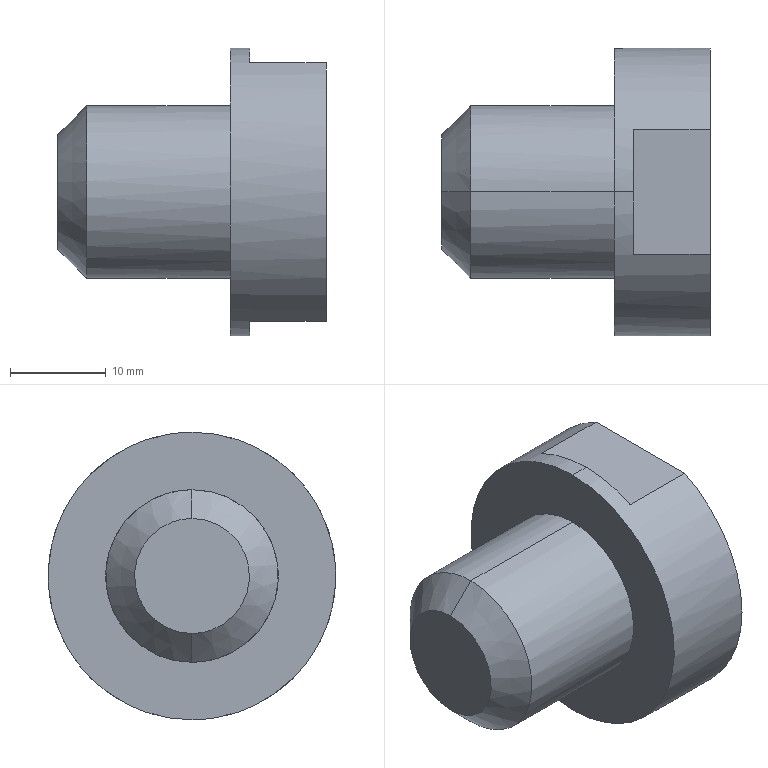Part | SolidWorks | features BaseBody 1 | 1 solid | 19 faces | box 28 x 30 x 30 mm | volume 9162 mm3 | plane 7 | cone 6 | cylinder 6 | commonest cylinder face diameters 10.106 x2 18 x2 30 x2
STEP:
#1=CARTESIAN_POINT('',(26.5,0.,5.053));
#2=VERTEX_POINT('',#1);
#3=CARTESIAN_POINT('',(26.5,0.,-5.053));
#4=VERTEX_POINT('',#3);
#5=CARTESIAN_POINT('',(26.5,0.,5.053));
#6=CARTESIAN_POINT('',(26.5,-0.6614,5.053));
#7=CARTESIAN_POINT('',(26.5,-1.323,4.921));
#8=CARTESIAN_POINT('',(26.5,-2.545,4.415));
#9=CARTESIAN_POINT('',(26.5,-3.105,4.041));
#10=CARTESIAN_POINT('',(26.5,-4.041,3.105));
#11=CARTESIAN_POINT('',(26.5,-4.415,2.545));
#12=CARTESIAN_POINT('',(26.5,-4.921,1.323));
#13=CARTESIAN_POINT('',(26.5,-5.053,0.6614));
#14=CARTESIAN_POINT('',(26.5,-5.053,-0.6614));
#15=CARTESIAN_POINT('',(26.5,-4.921,-1.323));
#16=CARTESIAN_POINT('',(26.5,-4.415,-2.545));
#17=CARTESIAN_POINT('',(26.5,-4.041,-3.105));
#18=CARTESIAN_POINT('',(26.5,-3.105,-4.041));
#19=CARTESIAN_POINT('',(26.5,-2.545,-4.415));
#20=CARTESIAN_POINT('',(26.5,-1.323,-4.921));
#21=CARTESIAN_POINT('',(26.5,-0.6614,-5.053));
#22=CARTESIAN_POINT('',(26.5,0.,-5.053));
#23=B_SPLINE_CURVE_WITH_KNOTS('',3,(#5,#6,#7,#8,#9,#10,#11,#12,#13,#14,#15,#16,#17,#18,#19,#20,#21,#22),.UNSPECIFIED.,.F.,.F.,(4,2,2,2,2,2,2,2,4),(3.142,3.534,3.927,4.32,4.712,5.105,5.498,5.89,6.283),.UNSPECIFIED.);
#24=EDGE_CURVE('',#2,#4,#23,.T.);
#25=ORIENTED_EDGE('',*,*,#24,.F.);
#26=CARTESIAN_POINT('',(28.,0.,6.553));
#27=VERTEX_POINT('',#26);
#28=CARTESIAN_POINT('',(26.5,0.,5.053));
#29=DIRECTION('',(0.7071,0.,0.7071));
#30=VECTOR('',#29,1000.);
#31=LINE('',#28,#30);
#32=EDGE_CURVE('',#2,#27,#31,.T.);
#33=ORIENTED_EDGE('',*,*,#32,.T.);
#34=CARTESIAN_POINT('',(28.,0.,-6.553));
#35=VERTEX_POINT('',#34);
#36=CARTESIAN_POINT('',(28.,0.,6.553));
#37=CARTESIAN_POINT('',(28.,-0.8578,6.553));
#38=CARTESIAN_POINT('',(28.,-1.715,6.382));
#39=CARTESIAN_POINT('',(28.,-3.3,5.726));
#40=CARTESIAN_POINT('',(28.,-4.027,5.24));
#41=CARTESIAN_POINT('',(28.,-5.24,4.027));
#42=CARTESIAN_POINT('',(28.,-5.726,3.3));
#43=CARTESIAN_POINT('',(28.,-6.382,1.715));
#44=CARTESIAN_POINT('',(28.,-6.553,0.8578));
#45=CARTESIAN_POINT('',(28.,-6.553,-0.8578));
#46=CARTESIAN_POINT('',(28.,-6.382,-1.715));
#47=CARTESIAN_POINT('',(28.,-5.726,-3.3));
#48=CARTESIAN_POINT('',(28.,-5.24,-4.027));
#49=CARTESIAN_POINT('',(28.,-4.027,-5.24));
#50=CARTESIAN_POINT('',(28.,-3.3,-5.726));
#51=CARTESIAN_POINT('',(28.,-1.715,-6.382));
#52=CARTESIAN_POINT('',(28.,-0.8578,-6.553));
#53=CARTESIAN_POINT('',(28.,0.,-6.553));
#54=B_SPLINE_CURVE_WITH_KNOTS('',3,(#36,#37,#38,#39,#40,#41,#42,#43,#44,#45,#46,#47,#48,#49,#50,#51,#52,#53),.UNSPECIFIED.,.F.,.F.,(4,2,2,2,2,2,2,2,4),(3.142,3.534,3.927,4.32,4.712,5.105,5.498,5.89,6.283),.UNSPECIFIED.);
#55=EDGE_CURVE('',#27,#35,#54,.T.);
#56=ORIENTED_EDGE('',*,*,#55,.T.);
#57=CARTESIAN_POINT('',(26.5,0.,-5.053));
#58=DIRECTION('',(0.7071,0.,-0.7071));
#59=VECTOR('',#58,1000.);
#60=LINE('',#57,#59);
#61=EDGE_CURVE('',#4,#35,#60,.T.);
#62=ORIENTED_EDGE('',*,*,#61,.F.);
#63=EDGE_LOOP('',(#25,#33,#56,#62));
#64=FACE_OUTER_BOUND('',#63,.T.);
#65=CARTESIAN_POINT('',(26.5,0.,0.));
#66=DIRECTION('',(1.,0.,0.));
#67=DIRECTION('',(0.,0.,-1.));
#68=AXIS2_PLACEMENT_3D('',#65,#66,#67);
#69=CONICAL_SURFACE('',#68,5.053,0.7854);
#70=ADVANCED_FACE('',(#64),#69,.F.);
#71=CARTESIAN_POINT('',(3.917,0.,5.053));
#72=VERTEX_POINT('',#71);
#73=CARTESIAN_POINT('',(3.917,0.,-5.053));
#74=VERTEX_POINT('',#73);
#75=CARTESIAN_POINT('',(3.917,0.,5.053));
#76=CARTESIAN_POINT('',(3.917,-0.6614,5.053));
#77=CARTESIAN_POINT('',(3.917,-1.323,4.921));
#78=CARTESIAN_POINT('',(3.917,-2.545,4.415));
#79=CARTESIAN_POINT('',(3.917,-3.105,4.041));
#80=CARTESIAN_POINT('',(3.917,-4.041,3.105));
#81=CARTESIAN_POINT('',(3.917,-4.415,2.545));
#82=CARTESIAN_POINT('',(3.917,-4.921,1.323));
#83=CARTESIAN_POINT('',(3.917,-5.053,0.6614));
#84=CARTESIAN_POINT('',(3.917,-5.053,-0.6614));
#85=CARTESIAN_POINT('',(3.917,-4.921,-1.323));
#86=CARTESIAN_POINT('',(3.917,-4.415,-2.545));
#87=CARTESIAN_POINT('',(3.917,-4.041,-3.105));
#88=CARTESIAN_POINT('',(3.917,-3.105,-4.041));
#89=CARTESIAN_POINT('',(3.917,-2.545,-4.415));
#90=CARTESIAN_POINT('',(3.917,-1.323,-4.921));
#91=CARTESIAN_POINT('',(3.917,-0.6614,-5.053));
#92=CARTESIAN_POINT('',(3.917,0.,-5.053));
#93=B_SPLINE_CURVE_WITH_KNOTS('',3,(#75,#76,#77,#78,#79,#80,#81,#82,#83,#84,#85,#86,#87,#88,#89,#90,#91,#92),.UNSPECIFIED.,.F.,.F.,(4,2,2,2,2,2,2,2,4),(3.142,3.534,3.927,4.32,4.712,5.105,5.498,5.89,6.283),.UNSPECIFIED.);
#94=EDGE_CURVE('',#72,#74,#93,.T.);
#95=ORIENTED_EDGE('',*,*,#94,.F.);
#96=CARTESIAN_POINT('',(28.,0.,5.053));
#97=DIRECTION('',(1.,0.,0.));
#98=VECTOR('',#97,1000.);
#99=LINE('',#96,#98);
#100=EDGE_CURVE('',#72,#2,#99,.T.);
#101=ORIENTED_EDGE('',*,*,#100,.T.);
#102=ORIENTED_EDGE('',*,*,#24,.T.);
#103=CARTESIAN_POINT('',(28.,0.,-5.053));
#104=DIRECTION('',(1.,0.,0.));
#105=VECTOR('',#104,1000.);
#106=LINE('',#103,#105);
#107=EDGE_CURVE('',#74,#4,#106,.T.);
#108=ORIENTED_EDGE('',*,*,#107,.F.);
#109=EDGE_LOOP('',(#95,#101,#102,#108));
#110=FACE_OUTER_BOUND('',#109,.T.);
#111=CARTESIAN_POINT('',(28.,0.,0.));
#112=DIRECTION('',(1.,0.,0.));
#113=DIRECTION('',(0.,0.,-1.));
#114=AXIS2_PLACEMENT_3D('',#111,#112,#113);
#115=CYLINDRICAL_SURFACE('',#114,5.053);
#116=ADVANCED_FACE('',(#110),#115,.F.);
#117=CARTESIAN_POINT('',(1.,0.,0.));
#118=VERTEX_POINT('',#117);
#119=CARTESIAN_POINT('',(1.,0.,0.));
#120=DIRECTION('',(0.5,0.,-0.866));
#121=VECTOR('',#120,1000.);
#122=LINE('',#119,#121);
#123=EDGE_CURVE('',#118,#74,#122,.T.);
#124=ORIENTED_EDGE('',*,*,#123,.F.);
#125=CARTESIAN_POINT('',(1.,0.,0.));
#126=DIRECTION('',(0.5,0.,0.866));
#127=VECTOR('',#126,1000.);
#128=LINE('',#125,#127);
#129=EDGE_CURVE('',#118,#72,#128,.T.);
#130=ORIENTED_EDGE('',*,*,#129,.T.);
#131=ORIENTED_EDGE('',*,*,#94,.T.);
#132=EDGE_LOOP('',(#124,#130,#131));
#133=FACE_OUTER_BOUND('',#132,.T.);
#134=CARTESIAN_POINT('',(1001.,0.,0.));
#135=DIRECTION('',(1.,0.,0.));
#136=DIRECTION('',(0.,0.,-1.));
#137=AXIS2_PLACEMENT_3D('',#134,#135,#136);
#138=CONICAL_SURFACE('',#137,1732.051,1.047);
#139=ADVANCED_FACE('',(#133),#138,.F.);
#140=CARTESIAN_POINT('',(3.,0.,-9.));
#141=VERTEX_POINT('',#140);
#142=CARTESIAN_POINT('',(3.,0.,9.));
#143=VERTEX_POINT('',#142);
#144=CARTESIAN_POINT('',(3.,0.,-9.));
#145=CARTESIAN_POINT('',(3.,1.178,-9.));
#146=CARTESIAN_POINT('',(3.,2.356,-8.766));
#147=CARTESIAN_POINT('',(3.,4.533,-7.864));
#148=CARTESIAN_POINT('',(3.,5.531,-7.197));
#149=CARTESIAN_POINT('',(3.,7.197,-5.531));
#150=CARTESIAN_POINT('',(3.,7.864,-4.533));
#151=CARTESIAN_POINT('',(3.,8.766,-2.356));
#152=CARTESIAN_POINT('',(3.,9.,-1.178));
#153=CARTESIAN_POINT('',(3.,9.,1.178));
#154=CARTESIAN_POINT('',(3.,8.766,2.356));
#155=CARTESIAN_POINT('',(3.,7.864,4.533));
#156=CARTESIAN_POINT('',(3.,7.197,5.531));
#157=CARTESIAN_POINT('',(3.,5.531,7.197));
#158=CARTESIAN_POINT('',(3.,4.533,7.864));
#159=CARTESIAN_POINT('',(3.,2.356,8.766));
#160=CARTESIAN_POINT('',(3.,1.178,9.));
#161=CARTESIAN_POINT('',(3.,0.,9.));
#162=B_SPLINE_CURVE_WITH_KNOTS('',3,(#144,#145,#146,#147,#148,#149,#150,#151,#152,#153,#154,#155,#156,#157,#158,#159,#160,#161),.UNSPECIFIED.,.F.,.F.,(4,2,2,2,2,2,2,2,4),(0.,0.3927,0.7854,1.178,1.571,1.963,2.356,2.749,3.142),.UNSPECIFIED.);
#163=EDGE_CURVE('',#141,#143,#162,.T.);
#164=ORIENTED_EDGE('',*,*,#163,.T.);
#165=CARTESIAN_POINT('',(18.,0.,9.));
#166=VERTEX_POINT('',#165);
#167=CARTESIAN_POINT('',(28.,0.,9.));
#168=DIRECTION('',(1.,0.,0.));
#169=VECTOR('',#168,1000.);
#170=LINE('',#167,#169);
#171=EDGE_CURVE('',#143,#166,#170,.T.);
#172=ORIENTED_EDGE('',*,*,#171,.T.);
#173=CARTESIAN_POINT('',(18.,0.,-9.));
#174=VERTEX_POINT('',#173);
#175=CARTESIAN_POINT('',(18.,0.,-9.));
#176=CARTESIAN_POINT('',(18.,0.5909,-9.));
#177=CARTESIAN_POINT('',(18.,1.176,-8.942));
#178=CARTESIAN_POINT('',(18.,2.335,-8.712));
#179=CARTESIAN_POINT('',(18.,2.898,-8.541));
#180=CARTESIAN_POINT('',(18.,3.99,-8.089));
#181=CARTESIAN_POINT('',(18.,4.509,-7.812));
#182=CARTESIAN_POINT('',(18.,5.491,-7.155));
#183=CARTESIAN_POINT('',(18.,5.946,-6.782));
#184=CARTESIAN_POINT('',(18.,6.782,-5.946));
#185=CARTESIAN_POINT('',(18.,7.155,-5.491));
#186=CARTESIAN_POINT('',(18.,7.812,-4.509));
#187=CARTESIAN_POINT('',(18.,8.089,-3.99));
#188=CARTESIAN_POINT('',(18.,8.541,-2.898));
#189=CARTESIAN_POINT('',(18.,8.712,-2.335));
#190=CARTESIAN_POINT('',(18.,8.942,-1.176));
#191=CARTESIAN_POINT('',(18.,9.,-0.5909));
#192=CARTESIAN_POINT('',(18.,9.,0.5909));
#193=CARTESIAN_POINT('',(18.,8.942,1.176));
#194=CARTESIAN_POINT('',(18.,8.712,2.335));
#195=CARTESIAN_POINT('',(18.,8.541,2.898));
#196=CARTESIAN_POINT('',(18.,8.089,3.99));
#197=CARTESIAN_POINT('',(18.,7.812,4.509));
#198=CARTESIAN_POINT('',(18.,7.155,5.491));
#199=CARTESIAN_POINT('',(18.,6.782,5.946));
#200=CARTESIAN_POINT('',(18.,5.946,6.782));
#201=CARTESIAN_POINT('',(18.,5.491,7.155));
#202=CARTESIAN_POINT('',(18.,4.509,7.812));
#203=CARTESIAN_POINT('',(18.,3.99,8.089));
#204=CARTESIAN_POINT('',(18.,2.898,8.541));
#205=CARTESIAN_POINT('',(18.,2.335,8.712));
#206=CARTESIAN_POINT('',(18.,1.176,8.942));
#207=CARTESIAN_POINT('',(18.,0.5909,9.));
#208=CARTESIAN_POINT('',(18.,0.,9.));
#209=B_SPLINE_CURVE_WITH_KNOTS('',3,(#175,#176,#177,#178,#179,#180,#181,#182,#183,#184,#185,#186,#187,#188,#189,#190,#191,#192,#193,#194,#195,#196,#197,#198,#199,#200,#201,#202,#203,#204,#205,#206,#207,#208),.UNSPECIFIED.,.F.,.F.,(4,2,2,2,2,2,2,2,2,2,2,2,2,2,2,2,4),(0.,0.1963,0.3927,0.589,0.7854,0.9817,1.178,1.374,1.571,1.767,1.963,2.16,2.356,2.553,2.749,2.945,3.142),.UNSPECIFIED.);
#210=EDGE_CURVE('',#174,#166,#209,.T.);
#211=ORIENTED_EDGE('',*,*,#210,.F.);
#212=CARTESIAN_POINT('',(28.,0.,-9.));
#213=DIRECTION('',(1.,0.,0.));
#214=VECTOR('',#213,1000.);
#215=LINE('',#212,#214);
#216=EDGE_CURVE('',#141,#174,#215,.T.);
#217=ORIENTED_EDGE('',*,*,#216,.F.);
#218=EDGE_LOOP('',(#164,#172,#211,#217));
#219=FACE_OUTER_BOUND('',#218,.T.);
#220=CARTESIAN_POINT('',(28.,0.,0.));
#221=DIRECTION('',(1.,0.,0.));
#222=DIRECTION('',(0.,0.,-1.));
#223=AXIS2_PLACEMENT_3D('',#220,#221,#222);
#224=CYLINDRICAL_SURFACE('',#223,9.);
#225=ADVANCED_FACE('',(#219),#224,.T.);
#226=CARTESIAN_POINT('',(0.,0.,-6.));
#227=VERTEX_POINT('',#226);
#228=CARTESIAN_POINT('',(0.,0.,6.));
#229=VERTEX_POINT('',#228);
#230=CARTESIAN_POINT('',(0.,0.,-6.));
#231=CARTESIAN_POINT('',(0.,0.7854,-6.));
#232=CARTESIAN_POINT('',(0.,1.57,-5.844));
#233=CARTESIAN_POINT('',(0.,3.022,-5.243));
#234=CARTESIAN_POINT('',(0.,3.687,-4.798));
#235=CARTESIAN_POINT('',(0.,4.798,-3.687));
#236=CARTESIAN_POINT('',(0.,5.243,-3.022));
#237=CARTESIAN_POINT('',(0.,5.844,-1.57));
#238=CARTESIAN_POINT('',(0.,6.,-0.7854));
#239=CARTESIAN_POINT('',(0.,6.,0.7854));
#240=CARTESIAN_POINT('',(0.,5.844,1.57));
#241=CARTESIAN_POINT('',(0.,5.243,3.022));
#242=CARTESIAN_POINT('',(0.,4.798,3.687));
#243=CARTESIAN_POINT('',(0.,3.687,4.798));
#244=CARTESIAN_POINT('',(0.,3.022,5.243));
#245=CARTESIAN_POINT('',(0.,1.57,5.844));
#246=CARTESIAN_POINT('',(0.,0.7854,6.));
#247=CARTESIAN_POINT('',(0.,0.,6.));
#248=B_SPLINE_CURVE_WITH_KNOTS('',3,(#230,#231,#232,#233,#234,#235,#236,#237,#238,#239,#240,#241,#242,#243,#244,#245,#246,#247),.UNSPECIFIED.,.F.,.F.,(4,2,2,2,2,2,2,2,4),(0.,0.3927,0.7854,1.178,1.571,1.963,2.356,2.749,3.142),.UNSPECIFIED.);
#249=EDGE_CURVE('',#227,#229,#248,.T.);
#250=ORIENTED_EDGE('',*,*,#249,.T.);
#251=CARTESIAN_POINT('',(0.,0.,6.));
#252=DIRECTION('',(0.7071,0.,0.7071));
#253=VECTOR('',#252,1000.);
#254=LINE('',#251,#253);
#255=EDGE_CURVE('',#229,#143,#254,.T.);
#256=ORIENTED_EDGE('',*,*,#255,.T.);
#257=ORIENTED_EDGE('',*,*,#163,.F.);
#258=CARTESIAN_POINT('',(0.,0.,-6.));
#259=DIRECTION('',(0.7071,0.,-0.7071));
#260=VECTOR('',#259,1000.);
#261=LINE('',#258,#260);
#262=EDGE_CURVE('',#227,#141,#261,.T.);
#263=ORIENTED_EDGE('',*,*,#262,.F.);
#264=EDGE_LOOP('',(#250,#256,#257,#263));
#265=FACE_OUTER_BOUND('',#264,.T.);
#266=CARTESIAN_POINT('',(0.,0.,0.));
#267=DIRECTION('',(1.,0.,0.));
#268=DIRECTION('',(0.,0.,-1.));
#269=AXIS2_PLACEMENT_3D('',#266,#267,#268);
#270=CONICAL_SURFACE('',#269,6.,0.7854);
#271=ADVANCED_FACE('',(#265),#270,.T.);
#272=CARTESIAN_POINT('',(18.,0.,-15.));
#273=VERTEX_POINT('',#272);
#274=CARTESIAN_POINT('',(18.,0.,15.));
#275=VERTEX_POINT('',#274);
#276=CARTESIAN_POINT('',(18.,0.,-15.));
#277=CARTESIAN_POINT('',(18.,1.963,-15.));
#278=CARTESIAN_POINT('',(18.,3.926,-14.61));
#279=CARTESIAN_POINT('',(18.,7.554,-13.107));
#280=CARTESIAN_POINT('',(18.,9.218,-11.995));
#281=CARTESIAN_POINT('',(18.,11.995,-9.218));
#282=CARTESIAN_POINT('',(18.,13.107,-7.554));
#283=CARTESIAN_POINT('',(18.,14.61,-3.926));
#284=CARTESIAN_POINT('',(18.,15.,-1.963));
#285=CARTESIAN_POINT('',(18.,15.,1.963));
#286=CARTESIAN_POINT('',(18.,14.61,3.926));
#287=CARTESIAN_POINT('',(18.,13.107,7.554));
#288=CARTESIAN_POINT('',(18.,11.995,9.218));
#289=CARTESIAN_POINT('',(18.,9.218,11.995));
#290=CARTESIAN_POINT('',(18.,7.554,13.107));
#291=CARTESIAN_POINT('',(18.,3.926,14.61));
#292=CARTESIAN_POINT('',(18.,1.963,15.));
#293=CARTESIAN_POINT('',(18.,0.,15.));
#294=B_SPLINE_CURVE_WITH_KNOTS('',3,(#276,#277,#278,#279,#280,#281,#282,#283,#284,#285,#286,#287,#288,#289,#290,#291,#292,#293),.UNSPECIFIED.,.F.,.F.,(4,2,2,2,2,2,2,2,4),(0.,0.3927,0.7854,1.178,1.571,1.963,2.356,2.749,3.142),.UNSPECIFIED.);
#295=EDGE_CURVE('',#273,#275,#294,.T.);
#296=ORIENTED_EDGE('',*,*,#295,.T.);
#297=CARTESIAN_POINT('',(20.,0.,15.));
#298=VERTEX_POINT('',#297);
#299=CARTESIAN_POINT('',(28.,0.,15.));
#300=DIRECTION('',(1.,0.,0.));
#301=VECTOR('',#300,1000.);
#302=LINE('',#299,#301);
#303=EDGE_CURVE('',#275,#298,#302,.T.);
#304=ORIENTED_EDGE('',*,*,#303,.T.);
#305=CARTESIAN_POINT('',(20.,6.538,13.5));
#306=VERTEX_POINT('',#305);
#307=CARTESIAN_POINT('',(20.,0.,0.));
#308=DIRECTION('',(1.,0.,0.));
#309=DIRECTION('',(0.,0.4359,0.9));
#310=AXIS2_PLACEMENT_3D('',#307,#308,#309);
#311=CIRCLE('',#310,15.);
#312=EDGE_CURVE('',#306,#298,#311,.T.);
#313=ORIENTED_EDGE('',*,*,#312,.F.);
#314=CARTESIAN_POINT('',(28.,6.538,13.5));
#315=VERTEX_POINT('',#314);
#316=CARTESIAN_POINT('',(28.,6.538,13.5));
#317=DIRECTION('',(-1.,0.,0.));
#318=VECTOR('',#317,1000.);
#319=LINE('',#316,#318);
#320=EDGE_CURVE('',#315,#306,#319,.T.);
#321=ORIENTED_EDGE('',*,*,#320,.F.);
#322=CARTESIAN_POINT('',(28.,6.538,-13.5));
#323=VERTEX_POINT('',#322);
#324=CARTESIAN_POINT('',(28.,0.,0.));
#325=DIRECTION('',(1.,0.,0.));
#326=DIRECTION('',(0.,0.4359,-0.9));
#327=AXIS2_PLACEMENT_3D('',#324,#325,#326);
#328=CIRCLE('',#327,15.);
#329=EDGE_CURVE('',#323,#315,#328,.T.);
#330=ORIENTED_EDGE('',*,*,#329,.F.);
#331=CARTESIAN_POINT('',(20.,6.538,-13.5));
#332=VERTEX_POINT('',#331);
#333=CARTESIAN_POINT('',(20.,6.538,-13.5));
#334=DIRECTION('',(1.,0.,0.));
#335=VECTOR('',#334,1000.);
#336=LINE('',#333,#335);
#337=EDGE_CURVE('',#332,#323,#336,.T.);
#338=ORIENTED_EDGE('',*,*,#337,.F.);
#339=CARTESIAN_POINT('',(20.,0.,-15.));
#340=VERTEX_POINT('',#339);
#341=CARTESIAN_POINT('',(20.,0.,0.));
#342=DIRECTION('',(1.,0.,0.));
#343=DIRECTION('',(0.,-0.4359,-0.9));
#344=AXIS2_PLACEMENT_3D('',#341,#342,#343);
#345=CIRCLE('',#344,15.);
#346=EDGE_CURVE('',#340,#332,#345,.T.);
#347=ORIENTED_EDGE('',*,*,#346,.F.);
#348=CARTESIAN_POINT('',(28.,0.,-15.));
#349=DIRECTION('',(1.,0.,0.));
#350=VECTOR('',#349,1000.);
#351=LINE('',#348,#350);
#352=EDGE_CURVE('',#273,#340,#351,.T.);
#353=ORIENTED_EDGE('',*,*,#352,.F.);
#354=EDGE_LOOP('',(#296,#304,#313,#321,#330,#338,#347,#353));
#355=FACE_OUTER_BOUND('',#354,.T.);
#356=CARTESIAN_POINT('',(28.,0.,0.));
#357=DIRECTION('',(1.,0.,0.));
#358=DIRECTION('',(0.,0.,-1.));
#359=AXIS2_PLACEMENT_3D('',#356,#357,#358);
#360=CYLINDRICAL_SURFACE('',#359,15.);
#361=ADVANCED_FACE('',(#355),#360,.T.);
#362=ORIENTED_EDGE('',*,*,#303,.F.);
#363=CARTESIAN_POINT('',(18.,0.,15.));
#364=CARTESIAN_POINT('',(18.,-1.963,15.));
#365=CARTESIAN_POINT('',(18.,-3.926,14.61));
#366=CARTESIAN_POINT('',(18.,-7.554,13.107));
#367=CARTESIAN_POINT('',(18.,-9.218,11.995));
#368=CARTESIAN_POINT('',(18.,-11.995,9.218));
#369=CARTESIAN_POINT('',(18.,-13.107,7.554));
#370=CARTESIAN_POINT('',(18.,-14.61,3.926));
#371=CARTESIAN_POINT('',(18.,-15.,1.963));
#372=CARTESIAN_POINT('',(18.,-15.,-1.963));
#373=CARTESIAN_POINT('',(18.,-14.61,-3.926));
#374=CARTESIAN_POINT('',(18.,-13.107,-7.554));
#375=CARTESIAN_POINT('',(18.,-11.995,-9.218));
#376=CARTESIAN_POINT('',(18.,-9.218,-11.995));
#377=CARTESIAN_POINT('',(18.,-7.554,-13.107));
#378=CARTESIAN_POINT('',(18.,-3.926,-14.61));
#379=CARTESIAN_POINT('',(18.,-1.963,-15.));
#380=CARTESIAN_POINT('',(18.,0.,-15.));
#381=B_SPLINE_CURVE_WITH_KNOTS('',3,(#363,#364,#365,#366,#367,#368,#369,#370,#371,#372,#373,#374,#375,#376,#377,#378,#379,#380),.UNSPECIFIED.,.F.,.F.,(4,2,2,2,2,2,2,2,4),(3.142,3.534,3.927,4.32,4.712,5.105,5.498,5.89,6.283),.UNSPECIFIED.);
#382=EDGE_CURVE('',#275,#273,#381,.T.);
#383=ORIENTED_EDGE('',*,*,#382,.T.);
#384=ORIENTED_EDGE('',*,*,#352,.T.);
#385=CARTESIAN_POINT('',(20.,-6.538,-13.5));
#386=VERTEX_POINT('',#385);
#387=CARTESIAN_POINT('',(20.,0.,0.));
#388=DIRECTION('',(1.,0.,0.));
#389=DIRECTION('',(0.,-0.4359,-0.9));
#390=AXIS2_PLACEMENT_3D('',#387,#388,#389);
#391=CIRCLE('',#390,15.);
#392=EDGE_CURVE('',#386,#340,#391,.T.);
#393=ORIENTED_EDGE('',*,*,#392,.F.);
#394=CARTESIAN_POINT('',(28.,-6.538,-13.5));
#395=VERTEX_POINT('',#394);
#396=CARTESIAN_POINT('',(28.,-6.538,-13.5));
#397=DIRECTION('',(-1.,0.,0.));
#398=VECTOR('',#397,1000.);
#399=LINE('',#396,#398);
#400=EDGE_CURVE('',#395,#386,#399,.T.);
#401=ORIENTED_EDGE('',*,*,#400,.F.);
#402=CARTESIAN_POINT('',(28.,-6.538,13.5));
#403=VERTEX_POINT('',#402);
#404=CARTESIAN_POINT('',(28.,0.,0.));
#405=DIRECTION('',(1.,0.,0.));
#406=DIRECTION('',(0.,-0.4359,0.9));
#407=AXIS2_PLACEMENT_3D('',#404,#405,#406);
#408=CIRCLE('',#407,15.);
#409=EDGE_CURVE('',#403,#395,#408,.T.);
#410=ORIENTED_EDGE('',*,*,#409,.F.);
#411=CARTESIAN_POINT('',(20.,-6.538,13.5));
#412=VERTEX_POINT('',#411);
#413=CARTESIAN_POINT('',(20.,-6.538,13.5));
#414=DIRECTION('',(1.,0.,0.));
#415=VECTOR('',#414,1000.);
#416=LINE('',#413,#415);
#417=EDGE_CURVE('',#412,#403,#416,.T.);
#418=ORIENTED_EDGE('',*,*,#417,.F.);
#419=CARTESIAN_POINT('',(20.,0.,0.));
#420=DIRECTION('',(1.,0.,0.));
#421=DIRECTION('',(0.,0.4359,0.9));
#422=AXIS2_PLACEMENT_3D('',#419,#420,#421);
#423=CIRCLE('',#422,15.);
#424=EDGE_CURVE('',#298,#412,#423,.T.);
#425=ORIENTED_EDGE('',*,*,#424,.F.);
#426=EDGE_LOOP('',(#362,#383,#384,#393,#401,#410,#418,#425));
#427=FACE_OUTER_BOUND('',#426,.T.);
#428=CARTESIAN_POINT('',(28.,0.,0.));
#429=DIRECTION('',(1.,0.,0.));
#430=DIRECTION('',(0.,0.,-1.));
#431=AXIS2_PLACEMENT_3D('',#428,#429,#430);
#432=CYLINDRICAL_SURFACE('',#431,15.);
#433=ADVANCED_FACE('',(#427),#432,.T.);
#434=CARTESIAN_POINT('',(28.,0.,-6.553));
#435=CARTESIAN_POINT('',(28.,0.8578,-6.553));
#436=CARTESIAN_POINT('',(28.,1.715,-6.382));
#437=CARTESIAN_POINT('',(28.,3.3,-5.726));
#438=CARTESIAN_POINT('',(28.,4.027,-5.24));
#439=CARTESIAN_POINT('',(28.,5.24,-4.027));
#440=CARTESIAN_POINT('',(28.,5.726,-3.3));
#441=CARTESIAN_POINT('',(28.,6.382,-1.715));
#442=CARTESIAN_POINT('',(28.,6.553,-0.8578));
#443=CARTESIAN_POINT('',(28.,6.553,0.8578));
#444=CARTESIAN_POINT('',(28.,6.382,1.715));
#445=CARTESIAN_POINT('',(28.,5.726,3.3));
#446=CARTESIAN_POINT('',(28.,5.24,4.027));
#447=CARTESIAN_POINT('',(28.,4.027,5.24));
#448=CARTESIAN_POINT('',(28.,3.3,5.726));
#449=CARTESIAN_POINT('',(28.,1.715,6.382));
#450=CARTESIAN_POINT('',(28.,0.8578,6.553));
#451=CARTESIAN_POINT('',(28.,0.,6.553));
#452=B_SPLINE_CURVE_WITH_KNOTS('',3,(#434,#435,#436,#437,#438,#439,#440,#441,#442,#443,#444,#445,#446,#447,#448,#449,#450,#451),.UNSPECIFIED.,.F.,.F.,(4,2,2,2,2,2,2,2,4),(0.,0.3927,0.7854,1.178,1.571,1.963,2.356,2.749,3.142),.UNSPECIFIED.);
#453=EDGE_CURVE('',#35,#27,#452,.T.);
#454=ORIENTED_EDGE('',*,*,#453,.F.);
#455=ORIENTED_EDGE('',*,*,#55,.F.);
#456=EDGE_LOOP('',(#454,#455));
#457=FACE_BOUND('',#456,.T.);
#458=CARTESIAN_POINT('',(28.,6.538,-13.5));
#459=DIRECTION('',(0.,-1.,0.));
#460=VECTOR('',#459,1000.);
#461=LINE('',#458,#460);
#462=EDGE_CURVE('',#323,#395,#461,.T.);
#463=ORIENTED_EDGE('',*,*,#462,.F.);
#464=ORIENTED_EDGE('',*,*,#329,.T.);
#465=CARTESIAN_POINT('',(28.,-6.538,13.5));
#466=DIRECTION('',(0.,1.,0.));
#467=VECTOR('',#466,1000.);
#468=LINE('',#465,#467);
#469=EDGE_CURVE('',#403,#315,#468,.T.);
#470=ORIENTED_EDGE('',*,*,#469,.F.);
#471=ORIENTED_EDGE('',*,*,#409,.T.);
#472=EDGE_LOOP('',(#463,#464,#470,#471));
#473=FACE_OUTER_BOUND('',#472,.T.);
#474=CARTESIAN_POINT('',(28.,15.,0.));
#475=DIRECTION('',(-1.,0.,0.));
#476=DIRECTION('',(0.,0.,1.));
#477=AXIS2_PLACEMENT_3D('',#474,#475,#476);
#478=PLANE('',#477);
#479=ADVANCED_FACE('',(#457,#473),#478,.F.);
#480=ORIENTED_EDGE('',*,*,#249,.F.);
#481=CARTESIAN_POINT('',(0.,0.,6.));
#482=CARTESIAN_POINT('',(0.,-0.7854,6.));
#483=CARTESIAN_POINT('',(0.,-1.57,5.844));
#484=CARTESIAN_POINT('',(0.,-3.022,5.243));
#485=CARTESIAN_POINT('',(0.,-3.687,4.798));
#486=CARTESIAN_POINT('',(0.,-4.798,3.687));
#487=CARTESIAN_POINT('',(0.,-5.243,3.022));
#488=CARTESIAN_POINT('',(0.,-5.844,1.57));
#489=CARTESIAN_POINT('',(0.,-6.,0.7854));
#490=CARTESIAN_POINT('',(0.,-6.,-0.7854));
#491=CARTESIAN_POINT('',(0.,-5.844,-1.57));
#492=CARTESIAN_POINT('',(0.,-5.243,-3.022));
#493=CARTESIAN_POINT('',(0.,-4.798,-3.687));
#494=CARTESIAN_POINT('',(0.,-3.687,-4.798));
#495=CARTESIAN_POINT('',(0.,-3.022,-5.243));
#496=CARTESIAN_POINT('',(0.,-1.57,-5.844));
#497=CARTESIAN_POINT('',(0.,-0.7854,-6.));
#498=CARTESIAN_POINT('',(0.,0.,-6.));
#499=B_SPLINE_CURVE_WITH_KNOTS('',3,(#481,#482,#483,#484,#485,#486,#487,#488,#489,#490,#491,#492,#493,#494,#495,#496,#497,#498),.UNSPECIFIED.,.F.,.F.,(4,2,2,2,2,2,2,2,4),(3.142,3.534,3.927,4.32,4.712,5.105,5.498,5.89,6.283),.UNSPECIFIED.);
#500=EDGE_CURVE('',#229,#227,#499,.T.);
#501=ORIENTED_EDGE('',*,*,#500,.F.);
#502=EDGE_LOOP('',(#480,#501));
#503=FACE_OUTER_BOUND('',#502,.T.);
#504=CARTESIAN_POINT('',(0.,0.,0.));
#505=DIRECTION('',(1.,0.,0.));
#506=DIRECTION('',(0.,0.,-1.));
#507=AXIS2_PLACEMENT_3D('',#504,#505,#506);
#508=PLANE('',#507);
#509=ADVANCED_FACE('',(#503),#508,.F.);
#510=ORIENTED_EDGE('',*,*,#255,.F.);
#511=ORIENTED_EDGE('',*,*,#500,.T.);
#512=ORIENTED_EDGE('',*,*,#262,.T.);
#513=CARTESIAN_POINT('',(3.,0.,9.));
#514=CARTESIAN_POINT('',(3.,-1.178,9.));
#515=CARTESIAN_POINT('',(3.,-2.356,8.766));
#516=CARTESIAN_POINT('',(3.,-4.533,7.864));
#517=CARTESIAN_POINT('',(3.,-5.531,7.197));
#518=CARTESIAN_POINT('',(3.,-7.197,5.531));
#519=CARTESIAN_POINT('',(3.,-7.864,4.533));
#520=CARTESIAN_POINT('',(3.,-8.766,2.356));
#521=CARTESIAN_POINT('',(3.,-9.,1.178));
#522=CARTESIAN_POINT('',(3.,-9.,-1.178));
#523=CARTESIAN_POINT('',(3.,-8.766,-2.356));
#524=CARTESIAN_POINT('',(3.,-7.864,-4.533));
#525=CARTESIAN_POINT('',(3.,-7.197,-5.531));
#526=CARTESIAN_POINT('',(3.,-5.531,-7.197));
#527=CARTESIAN_POINT('',(3.,-4.533,-7.864));
#528=CARTESIAN_POINT('',(3.,-2.356,-8.766));
#529=CARTESIAN_POINT('',(3.,-1.178,-9.));
#530=CARTESIAN_POINT('',(3.,0.,-9.));
#531=B_SPLINE_CURVE_WITH_KNOTS('',3,(#513,#514,#515,#516,#517,#518,#519,#520,#521,#522,#523,#524,#525,#526,#527,#528,#529,#530),.UNSPECIFIED.,.F.,.F.,(4,2,2,2,2,2,2,2,4),(3.142,3.534,3.927,4.32,4.712,5.105,5.498,5.89,6.283),.UNSPECIFIED.);
#532=EDGE_CURVE('',#143,#141,#531,.T.);
#533=ORIENTED_EDGE('',*,*,#532,.F.);
#534=EDGE_LOOP('',(#510,#511,#512,#533));
#535=FACE_OUTER_BOUND('',#534,.T.);
#536=CARTESIAN_POINT('',(0.,0.,0.));
#537=DIRECTION('',(1.,0.,0.));
#538=DIRECTION('',(0.,0.,-1.));
#539=AXIS2_PLACEMENT_3D('',#536,#537,#538);
#540=CONICAL_SURFACE('',#539,6.,0.7854);
#541=ADVANCED_FACE('',(#535),#540,.T.);
#542=ORIENTED_EDGE('',*,*,#171,.F.);
#543=ORIENTED_EDGE('',*,*,#532,.T.);
#544=ORIENTED_EDGE('',*,*,#216,.T.);
#545=CARTESIAN_POINT('',(18.,0.,9.));
#546=CARTESIAN_POINT('',(18.,-0.5909,9.));
#547=CARTESIAN_POINT('',(18.,-1.176,8.942));
#548=CARTESIAN_POINT('',(18.,-2.335,8.712));
#549=CARTESIAN_POINT('',(18.,-2.898,8.541));
#550=CARTESIAN_POINT('',(18.,-3.99,8.089));
#551=CARTESIAN_POINT('',(18.,-4.509,7.812));
#552=CARTESIAN_POINT('',(18.,-5.491,7.155));
#553=CARTESIAN_POINT('',(18.,-5.946,6.782));
#554=CARTESIAN_POINT('',(18.,-6.782,5.946));
#555=CARTESIAN_POINT('',(18.,-7.155,5.491));
#556=CARTESIAN_POINT('',(18.,-7.812,4.509));
#557=CARTESIAN_POINT('',(18.,-8.089,3.99));
#558=CARTESIAN_POINT('',(18.,-8.541,2.898));
#559=CARTESIAN_POINT('',(18.,-8.712,2.335));
#560=CARTESIAN_POINT('',(18.,-8.942,1.176));
#561=CARTESIAN_POINT('',(18.,-9.,0.5909));
#562=CARTESIAN_POINT('',(18.,-9.,-0.5909));
#563=CARTESIAN_POINT('',(18.,-8.942,-1.176));
#564=CARTESIAN_POINT('',(18.,-8.712,-2.335));
#565=CARTESIAN_POINT('',(18.,-8.541,-2.898));
#566=CARTESIAN_POINT('',(18.,-8.089,-3.99));
#567=CARTESIAN_POINT('',(18.,-7.812,-4.509));
#568=CARTESIAN_POINT('',(18.,-7.155,-5.491));
#569=CARTESIAN_POINT('',(18.,-6.782,-5.946));
#570=CARTESIAN_POINT('',(18.,-5.946,-6.782));
#571=CARTESIAN_POINT('',(18.,-5.491,-7.155));
#572=CARTESIAN_POINT('',(18.,-4.509,-7.812));
#573=CARTESIAN_POINT('',(18.,-3.99,-8.089));
#574=CARTESIAN_POINT('',(18.,-2.898,-8.541));
#575=CARTESIAN_POINT('',(18.,-2.335,-8.712));
#576=CARTESIAN_POINT('',(18.,-1.176,-8.942));
#577=CARTESIAN_POINT('',(18.,-0.5909,-9.));
#578=CARTESIAN_POINT('',(18.,0.,-9.));
#579=B_SPLINE_CURVE_WITH_KNOTS('',3,(#545,#546,#547,#548,#549,#550,#551,#552,#553,#554,#555,#556,#557,#558,#559,#560,#561,#562,#563,#564,#565,#566,#567,#568,#569,#570,#571,#572,#573,#574,#575,#576,#577,#578),.UNSPECIFIED.,.F.,.F.,(4,2,2,2,2,2,2,2,2,2,2,2,2,2,2,2,4),(3.142,3.338,3.534,3.731,3.927,4.123,4.32,4.516,4.712,4.909,5.105,5.301,5.498,5.694,5.89,6.087,6.283),.UNSPECIFIED.);
#580=EDGE_CURVE('',#166,#174,#579,.T.);
#581=ORIENTED_EDGE('',*,*,#580,.F.);
#582=EDGE_LOOP('',(#542,#543,#544,#581));
#583=FACE_OUTER_BOUND('',#582,.T.);
#584=CARTESIAN_POINT('',(28.,0.,0.));
#585=DIRECTION('',(1.,0.,0.));
#586=DIRECTION('',(0.,0.,-1.));
#587=AXIS2_PLACEMENT_3D('',#584,#585,#586);
#588=CYLINDRICAL_SURFACE('',#587,9.);
#589=ADVANCED_FACE('',(#583),#588,.T.);
#590=ORIENTED_EDGE('',*,*,#295,.F.);
#591=ORIENTED_EDGE('',*,*,#382,.F.);
#592=EDGE_LOOP('',(#590,#591));
#593=FACE_OUTER_BOUND('',#592,.T.);
#594=ORIENTED_EDGE('',*,*,#210,.T.);
#595=ORIENTED_EDGE('',*,*,#580,.T.);
#596=EDGE_LOOP('',(#594,#595));
#597=FACE_BOUND('',#596,.T.);
#598=CARTESIAN_POINT('',(18.,9.,0.));
#599=DIRECTION('',(1.,0.,0.));
#600=DIRECTION('',(0.,0.,-1.));
#601=AXIS2_PLACEMENT_3D('',#598,#599,#600);
#602=PLANE('',#601);
#603=ADVANCED_FACE('',(#593,#597),#602,.F.);
#604=ORIENTED_EDGE('',*,*,#129,.F.);
#605=ORIENTED_EDGE('',*,*,#123,.T.);
#606=CARTESIAN_POINT('',(3.917,0.,-5.053));
#607=CARTESIAN_POINT('',(3.917,0.6614,-5.053));
#608=CARTESIAN_POINT('',(3.917,1.323,-4.921));
#609=CARTESIAN_POINT('',(3.917,2.545,-4.415));
#610=CARTESIAN_POINT('',(3.917,3.105,-4.041));
#611=CARTESIAN_POINT('',(3.917,4.041,-3.105));
#612=CARTESIAN_POINT('',(3.917,4.415,-2.545));
#613=CARTESIAN_POINT('',(3.917,4.921,-1.323));
#614=CARTESIAN_POINT('',(3.917,5.053,-0.6614));
#615=CARTESIAN_POINT('',(3.917,5.053,0.6614));
#616=CARTESIAN_POINT('',(3.917,4.921,1.323));
#617=CARTESIAN_POINT('',(3.917,4.415,2.545));
#618=CARTESIAN_POINT('',(3.917,4.041,3.105));
#619=CARTESIAN_POINT('',(3.917,3.105,4.041));
#620=CARTESIAN_POINT('',(3.917,2.545,4.415));
#621=CARTESIAN_POINT('',(3.917,1.323,4.921));
#622=CARTESIAN_POINT('',(3.917,0.6614,5.053));
#623=CARTESIAN_POINT('',(3.917,0.,5.053));
#624=B_SPLINE_CURVE_WITH_KNOTS('',3,(#606,#607,#608,#609,#610,#611,#612,#613,#614,#615,#616,#617,#618,#619,#620,#621,#622,#623),.UNSPECIFIED.,.F.,.F.,(4,2,2,2,2,2,2,2,4),(0.,0.3927,0.7854,1.178,1.571,1.963,2.356,2.749,3.142),.UNSPECIFIED.);
#625=EDGE_CURVE('',#74,#72,#624,.T.);
#626=ORIENTED_EDGE('',*,*,#625,.T.);
#627=EDGE_LOOP('',(#604,#605,#626));
#628=FACE_OUTER_BOUND('',#627,.T.);
#629=CARTESIAN_POINT('',(1001.,0.,0.));
#630=DIRECTION('',(1.,0.,0.));
#631=DIRECTION('',(0.,0.,-1.));
#632=AXIS2_PLACEMENT_3D('',#629,#630,#631);
#633=CONICAL_SURFACE('',#632,1732.051,1.047);
#634=ADVANCED_FACE('',(#628),#633,.F.);
#635=ORIENTED_EDGE('',*,*,#100,.F.);
#636=ORIENTED_EDGE('',*,*,#625,.F.);
#637=ORIENTED_EDGE('',*,*,#107,.T.);
#638=CARTESIAN_POINT('',(26.5,0.,-5.053));
#639=CARTESIAN_POINT('',(26.5,0.6614,-5.053));
#640=CARTESIAN_POINT('',(26.5,1.323,-4.921));
#641=CARTESIAN_POINT('',(26.5,2.545,-4.415));
#642=CARTESIAN_POINT('',(26.5,3.105,-4.041));
#643=CARTESIAN_POINT('',(26.5,4.041,-3.105));
#644=CARTESIAN_POINT('',(26.5,4.415,-2.545));
#645=CARTESIAN_POINT('',(26.5,4.921,-1.323));
#646=CARTESIAN_POINT('',(26.5,5.053,-0.6614));
#647=CARTESIAN_POINT('',(26.5,5.053,0.6614));
#648=CARTESIAN_POINT('',(26.5,4.921,1.323));
#649=CARTESIAN_POINT('',(26.5,4.415,2.545));
#650=CARTESIAN_POINT('',(26.5,4.041,3.105));
#651=CARTESIAN_POINT('',(26.5,3.105,4.041));
#652=CARTESIAN_POINT('',(26.5,2.545,4.415));
#653=CARTESIAN_POINT('',(26.5,1.323,4.921));
#654=CARTESIAN_POINT('',(26.5,0.6614,5.053));
#655=CARTESIAN_POINT('',(26.5,0.,5.053));
#656=B_SPLINE_CURVE_WITH_KNOTS('',3,(#638,#639,#640,#641,#642,#643,#644,#645,#646,#647,#648,#649,#650,#651,#652,#653,#654,#655),.UNSPECIFIED.,.F.,.F.,(4,2,2,2,2,2,2,2,4),(0.,0.3927,0.7854,1.178,1.571,1.963,2.356,2.749,3.142),.UNSPECIFIED.);
#657=EDGE_CURVE('',#4,#2,#656,.T.);
#658=ORIENTED_EDGE('',*,*,#657,.T.);
#659=EDGE_LOOP('',(#635,#636,#637,#658));
#660=FACE_OUTER_BOUND('',#659,.T.);
#661=CARTESIAN_POINT('',(28.,0.,0.));
#662=DIRECTION('',(1.,0.,0.));
#663=DIRECTION('',(0.,0.,-1.));
#664=AXIS2_PLACEMENT_3D('',#661,#662,#663);
#665=CYLINDRICAL_SURFACE('',#664,5.053);
#666=ADVANCED_FACE('',(#660),#665,.F.);
#667=ORIENTED_EDGE('',*,*,#32,.F.);
#668=ORIENTED_EDGE('',*,*,#657,.F.);
#669=ORIENTED_EDGE('',*,*,#61,.T.);
#670=ORIENTED_EDGE('',*,*,#453,.T.);
#671=EDGE_LOOP('',(#667,#668,#669,#670));
#672=FACE_OUTER_BOUND('',#671,.T.);
#673=CARTESIAN_POINT('',(26.5,0.,0.));
#674=DIRECTION('',(1.,0.,0.));
#675=DIRECTION('',(0.,0.,-1.));
#676=AXIS2_PLACEMENT_3D('',#673,#674,#675);
#677=CONICAL_SURFACE('',#676,5.053,0.7854);
#678=ADVANCED_FACE('',(#672),#677,.F.);
#679=ORIENTED_EDGE('',*,*,#417,.T.);
#680=ORIENTED_EDGE('',*,*,#469,.T.);
#681=ORIENTED_EDGE('',*,*,#320,.T.);
#682=CARTESIAN_POINT('',(20.,6.538,13.5));
#683=DIRECTION('',(0.,-1.,0.));
#684=VECTOR('',#683,1000.);
#685=LINE('',#682,#684);
#686=EDGE_CURVE('',#306,#412,#685,.T.);
#687=ORIENTED_EDGE('',*,*,#686,.T.);
#688=EDGE_LOOP('',(#679,#680,#681,#687));
#689=FACE_OUTER_BOUND('',#688,.T.);
#690=CARTESIAN_POINT('',(20.,6.561,13.5));
#691=DIRECTION('',(0.,0.,1.));
#692=DIRECTION('',(1.,0.,0.));
#693=AXIS2_PLACEMENT_3D('',#690,#691,#692);
#694=PLANE('',#693);
#695=ADVANCED_FACE('',(#689),#694,.T.);
#696=ORIENTED_EDGE('',*,*,#312,.T.);
#697=ORIENTED_EDGE('',*,*,#424,.T.);
#698=ORIENTED_EDGE('',*,*,#686,.F.);
#699=EDGE_LOOP('',(#696,#697,#698));
#700=FACE_OUTER_BOUND('',#699,.T.);
#701=CARTESIAN_POINT('',(20.,0.,0.));
#702=DIRECTION('',(1.,0.,0.));
#703=DIRECTION('',(0.,0.,-1.));
#704=AXIS2_PLACEMENT_3D('',#701,#702,#703);
#705=PLANE('',#704);
#706=ADVANCED_FACE('',(#700),#705,.T.);
#707=ORIENTED_EDGE('',*,*,#392,.T.);
#708=ORIENTED_EDGE('',*,*,#346,.T.);
#709=CARTESIAN_POINT('',(20.,-6.538,-13.5));
#710=DIRECTION('',(0.,1.,0.));
#711=VECTOR('',#710,1000.);
#712=LINE('',#709,#711);
#713=EDGE_CURVE('',#386,#332,#712,.T.);
#714=ORIENTED_EDGE('',*,*,#713,.F.);
#715=EDGE_LOOP('',(#707,#708,#714));
#716=FACE_OUTER_BOUND('',#715,.T.);
#717=CARTESIAN_POINT('',(20.,0.,0.));
#718=DIRECTION('',(1.,0.,0.));
#719=DIRECTION('',(0.,0.,-1.));
#720=AXIS2_PLACEMENT_3D('',#717,#718,#719);
#721=PLANE('',#720);
#722=ADVANCED_FACE('',(#716),#721,.T.);
#723=ORIENTED_EDGE('',*,*,#337,.T.);
#724=ORIENTED_EDGE('',*,*,#462,.T.);
#725=ORIENTED_EDGE('',*,*,#400,.T.);
#726=ORIENTED_EDGE('',*,*,#713,.T.);
#727=EDGE_LOOP('',(#723,#724,#725,#726));
#728=FACE_OUTER_BOUND('',#727,.T.);
#729=CARTESIAN_POINT('',(20.,-6.561,-13.5));
#730=DIRECTION('',(0.,0.,-1.));
#731=DIRECTION('',(-1.,0.,0.));
#732=AXIS2_PLACEMENT_3D('',#729,#730,#731);
#733=PLANE('',#732);
#734=ADVANCED_FACE('',(#728),#733,.T.);
#735=CLOSED_SHELL('',(#70,#116,#139,#225,#271,#361,#433,#479,#509,#541,#589,#603,#634,#666,#678,#695,#706,#722,#734));
#736=MANIFOLD_SOLID_BREP('',#735);
#737=CARTESIAN_POINT('',(0.,0.,0.));
#738=DIRECTION('',(0.,0.,1.));
#739=DIRECTION('',(1.,0.,0.));
#740=AXIS2_PLACEMENT_3D('',#737,#738,#739);
#741=(LENGTH_UNIT()NAMED_UNIT(*)SI_UNIT(.MILLI.,.METRE.));
#742=UNCERTAINTY_MEASURE_WITH_UNIT(LENGTH_MEASURE(0.00001),#741,'','');
#743=(NAMED_UNIT(*)PLANE_ANGLE_UNIT()SI_UNIT($,.RADIAN.));
#744=(NAMED_UNIT(*)SI_UNIT($,.STERADIAN.)SOLID_ANGLE_UNIT());
#745=(GEOMETRIC_REPRESENTATION_CONTEXT(3)GLOBAL_UNCERTAINTY_ASSIGNED_CONTEXT((#742))GLOBAL_UNIT_ASSIGNED_CONTEXT((#741,#743,#744))REPRESENTATION_CONTEXT('',''));
#746=ADVANCED_BREP_SHAPE_REPRESENTATION('',(#736,#740),#745);